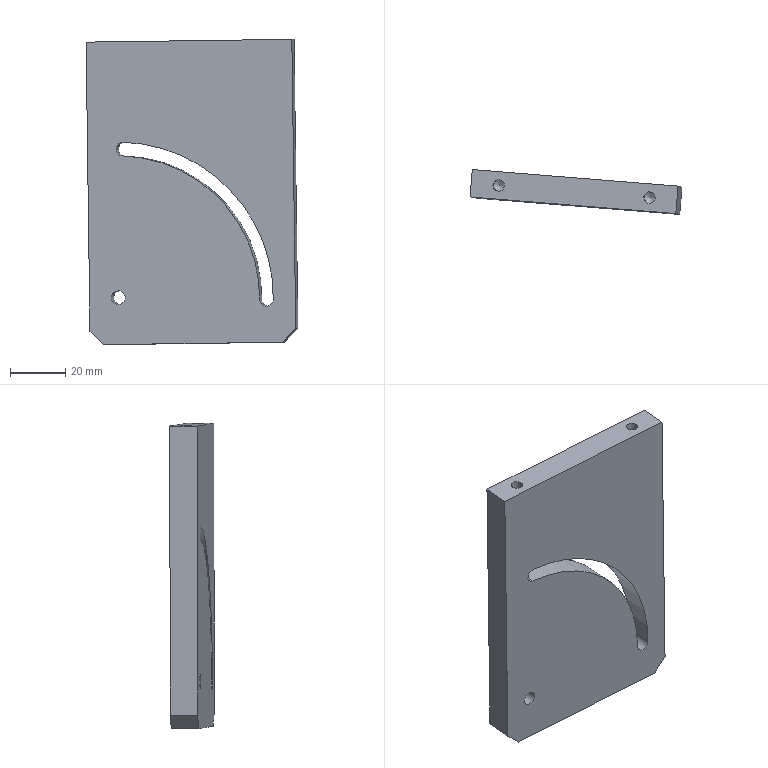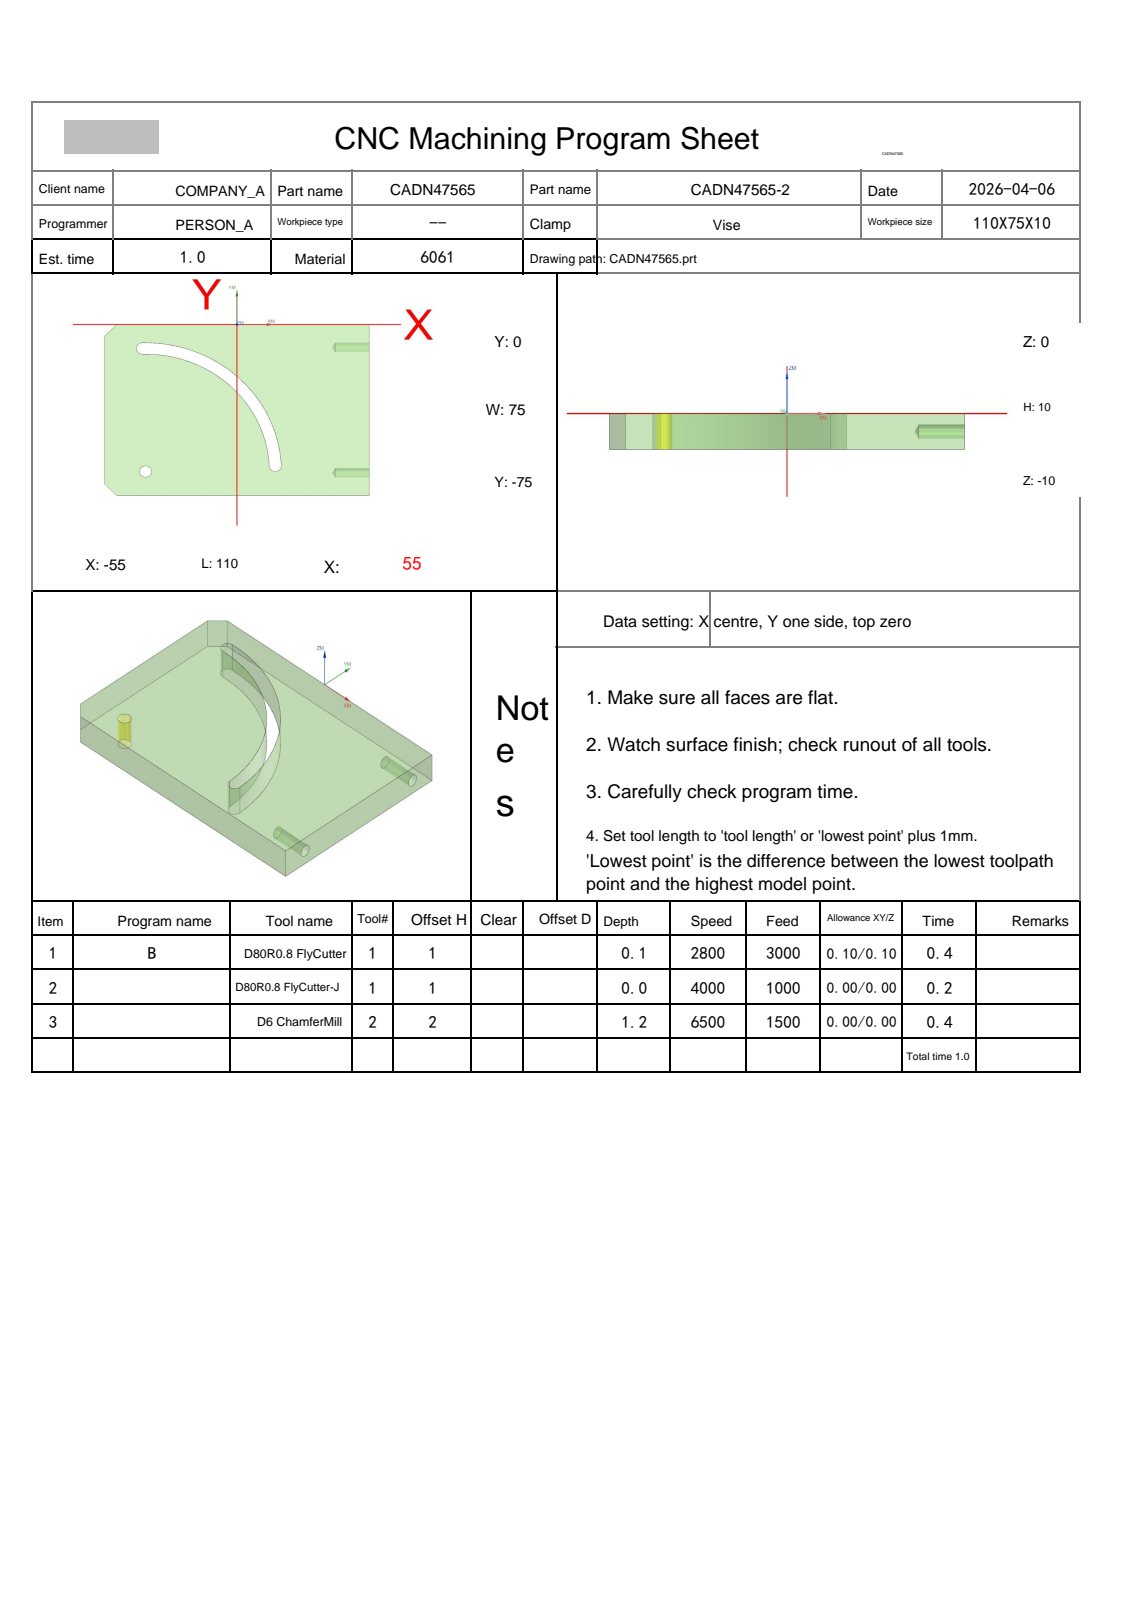NC program | NX | posted by the shop | part box 76.959 x 16.139 x 110.936 mm
Whole program:
%
O0001
(Machine time: 1.58 MIN)
(===Total Tool:2===)
(T1=D80R0.8 FlyCutter D=80.  R=0.8  D-  H01 Z=-0.   )
(T2=D6 ChamferMill D=6.   R=0.   D-  H02 Z=-1.2  )
G80 G90 G17 G49 G40
G91 G28 Z0
M01
N1 T01 M06
(D80R0.8 FlyCutter D=80. R=0.8 H=01 ce=0.10 di=0.10)
(MAX_Z=20. MIN_Z=0.1 Time=0.34M)
G00 G90 G54 X107.097 Y-37.5 M03 S2800
G43 H01 Z20.
M08
Z3.525
G01 Z1.525 F3000.
X95.097
X-95.097
X-107.097
Z3.525
G00 X107.097
Z3.05
G01 Z1.05
X95.097
X-95.097
X-107.097
Z3.05
G00 X107.097
Z2.575
G01 Z.575
X95.097
X-95.097
X-107.097
Z2.575
G00 X107.097
Z2.1
G01 Z.1
X95.097
X-95.097
X-107.097
Z2.1
G00 Z20.
G91 G28 Z0.0
M05
M09
G91 G28 Z0.0
M01
N2 T01 M06
(D80R0.8 FlyCutter-J D=80. R=0.8 H=01 ce=0.00 di=0.00)
(MAX_Z=20. MIN_Z=-0. Time=0.23M)
G00 G90 G54 X106.999 Y-37.5 M03 S4000
G43 H01 Z20.
M08
Z2.
G01 Z0.0 F1000.
X94.999
X-94.999
X-106.999
Z2.
G00 Z20.
G91 G28 Z0.0
M05
M09
G91 G28 Z0.0
M01
N3 T02 M06
(D6 ChamferMill D=6. R=0. H=02 ce=0.00 di=0.00)
(MAX_Z=20. MIN_Z=-1.2 Time=0.40M)
G00 G90 G54 X2.114 Y1.227 M03 S6500
G43 H02 Z20.
M08
Z.172
G01 Z-1.2 F1500.
G03 X2.4 Y1.027 I1.286 J1.532
G01 X2.446 Y.997
X2.5 Y1.
X55.
G02 X56. Y0.0 I0.0 J-1.
G01 Y-75.
G02 X55. Y-76. I-1. J0.0
G01 X-50.
X-50.259 Y-75.966
X-50.5 Y-75.866
X-50.707 Y-75.707
X-55.707 Y-70.707
X-55.866 Y-70.5
X-55.966 Y-70.259
X-56. Y-70.
Y-5.
X-55.966 Y-4.741
X-55.866 Y-4.5
X-55.707 Y-4.293
X-50.707 Y.707
X-50.5 Y.866
X-50.259 Y.966
X-50. Y1.
X2.5
X2.554 Y.997
X2.6 Y1.027
G03 X2.886 Y1.227 I-1. J1.732
G01 Z.172
G00 Z10.
X-.021 Y-24.33
Z.186
G01 Z-1.2
G03 X-.1 Y-23.99 I-1.98 J-.281
G01 X-.114 Y-23.937
X-.156 Y-23.903
G03 X-38. Y-9. I-37.844 J-40.597
X-39.323 Y-9.016 I0.0 J-55.5
X-40.787 Y-10.515 I.036 J-1.5
X-39.287 Y-12.015 I1.5 J0.0
G01 X-39.252
G02 X-38. Y-12. I1.252 J-52.485
X14.444 Y-62.069 I0.0 J-52.5
G03 X15.942 Y-63.5 I1.498 J.069
X17.442 Y-62. I0.0 J1.5
G01 X17.44 Y-61.93
G03 X-.156 Y-23.903 I-55.44 J-2.57
G01 X-.193 Y-23.863
X-.247 Y-23.853
G03 X-.591 Y-23.798 I-.485 J-1.94
G01 Z.186
G00 Z10.
X-39.32 Y-64.111
Z.284
G01 Z-1.2
G03 X-39.485 Y-64.418 I1.673 J-1.096
G01 X-39.509 Y-64.467
X-39.5 Y-64.52
G03 X-38. Y-66. I1.5 J.02
X-36.5 Y-64.5 I0.0 J1.5
X-38. Y-63. I-1.5 J0.0
X-39.5 Y-64.5 I0.0 J-1.5
G01 Y-64.52
X-39.508 Y-64.574
X-39.482 Y-64.622
G03 X-39.309 Y-64.925 I1.816 J.838
G01 Z.283
G00 Z20.
M05
M09
G91 G28 Z0.0
G91 G28 Y0.0
M30
%